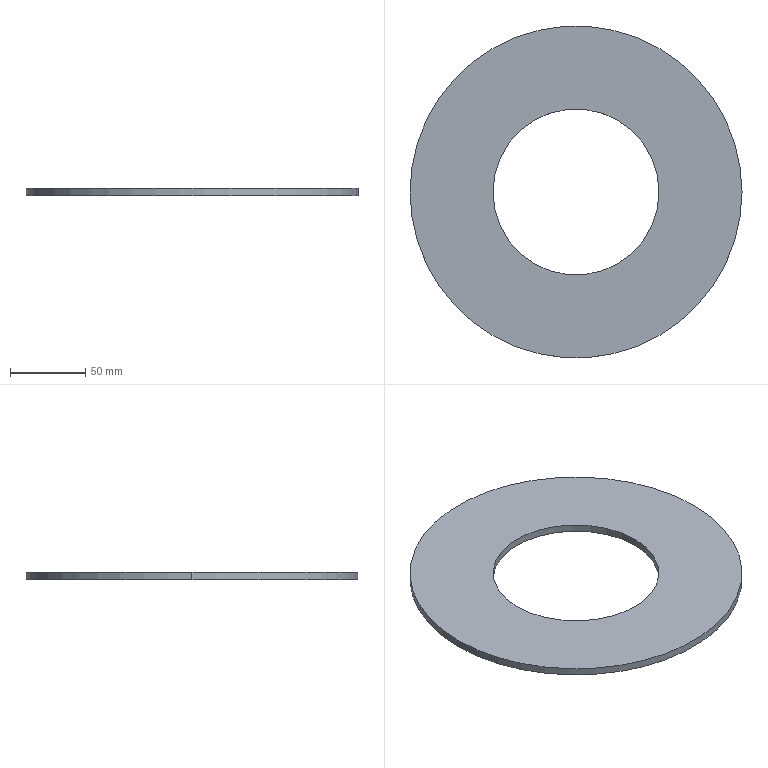Part | SolidWorks | features Extrusion 1 | 1 solid | 6 faces | box 220 x 220 x 5 mm | volume 142550 mm3 | cylinder 4 | plane 2 | commonest cylinder face diameters 110 x2 220 x2
STEP:
#1=CARTESIAN_POINT('',(-57.717,0.5838,5.));
#2=VERTEX_POINT('',#1);
#3=CARTESIAN_POINT('',(52.283,0.5838,5.));
#4=VERTEX_POINT('',#3);
#5=CARTESIAN_POINT('',(-2.717,0.5838,5.));
#6=DIRECTION('',(0.,0.,1.));
#7=DIRECTION('',(1.,0.,0.));
#8=AXIS2_PLACEMENT_3D('',#5,#6,#7);
#9=CIRCLE('',#8,55.);
#10=EDGE_CURVE('',#2,#4,#9,.T.);
#11=ORIENTED_EDGE('',*,*,#10,.T.);
#12=CARTESIAN_POINT('',(52.283,0.5838,0.));
#13=VERTEX_POINT('',#12);
#14=CARTESIAN_POINT('',(52.283,0.5838,5.));
#15=DIRECTION('',(0.,0.,-1.));
#16=VECTOR('',#15,1000.);
#17=LINE('',#14,#16);
#18=EDGE_CURVE('',#4,#13,#17,.T.);
#19=ORIENTED_EDGE('',*,*,#18,.T.);
#20=CARTESIAN_POINT('',(-57.717,0.5838,0.));
#21=VERTEX_POINT('',#20);
#22=CARTESIAN_POINT('',(-2.717,0.5838,0.));
#23=DIRECTION('',(0.,0.,1.));
#24=DIRECTION('',(1.,0.,0.));
#25=AXIS2_PLACEMENT_3D('',#22,#23,#24);
#26=CIRCLE('',#25,55.);
#27=EDGE_CURVE('',#21,#13,#26,.T.);
#28=ORIENTED_EDGE('',*,*,#27,.F.);
#29=CARTESIAN_POINT('',(-57.717,0.5838,5.));
#30=DIRECTION('',(0.,0.,-1.));
#31=VECTOR('',#30,1000.);
#32=LINE('',#29,#31);
#33=EDGE_CURVE('',#2,#21,#32,.T.);
#34=ORIENTED_EDGE('',*,*,#33,.F.);
#35=EDGE_LOOP('',(#11,#19,#28,#34));
#36=FACE_OUTER_BOUND('',#35,.T.);
#37=CARTESIAN_POINT('',(-2.717,0.5838,5.));
#38=DIRECTION('',(0.,0.,-1.));
#39=DIRECTION('',(-1.,0.,0.));
#40=AXIS2_PLACEMENT_3D('',#37,#38,#39);
#41=CYLINDRICAL_SURFACE('',#40,55.);
#42=ADVANCED_FACE('',(#36),#41,.F.);
#43=CARTESIAN_POINT('',(107.283,0.5838,5.));
#44=VERTEX_POINT('',#43);
#45=CARTESIAN_POINT('',(-112.717,0.5838,5.));
#46=VERTEX_POINT('',#45);
#47=CARTESIAN_POINT('',(-2.717,0.5838,5.));
#48=DIRECTION('',(0.,0.,1.));
#49=DIRECTION('',(1.,0.,0.));
#50=AXIS2_PLACEMENT_3D('',#47,#48,#49);
#51=CIRCLE('',#50,110.);
#52=EDGE_CURVE('',#44,#46,#51,.T.);
#53=ORIENTED_EDGE('',*,*,#52,.F.);
#54=CARTESIAN_POINT('',(107.283,0.5838,0.));
#55=VERTEX_POINT('',#54);
#56=CARTESIAN_POINT('',(107.283,0.5838,5.));
#57=DIRECTION('',(0.,0.,-1.));
#58=VECTOR('',#57,1000.);
#59=LINE('',#56,#58);
#60=EDGE_CURVE('',#44,#55,#59,.T.);
#61=ORIENTED_EDGE('',*,*,#60,.T.);
#62=CARTESIAN_POINT('',(-112.717,0.5838,0.));
#63=VERTEX_POINT('',#62);
#64=CARTESIAN_POINT('',(-2.717,0.5838,0.));
#65=DIRECTION('',(0.,0.,1.));
#66=DIRECTION('',(1.,0.,0.));
#67=AXIS2_PLACEMENT_3D('',#64,#65,#66);
#68=CIRCLE('',#67,110.);
#69=EDGE_CURVE('',#55,#63,#68,.T.);
#70=ORIENTED_EDGE('',*,*,#69,.T.);
#71=CARTESIAN_POINT('',(-112.717,0.5838,5.));
#72=DIRECTION('',(0.,0.,-1.));
#73=VECTOR('',#72,1000.);
#74=LINE('',#71,#73);
#75=EDGE_CURVE('',#46,#63,#74,.T.);
#76=ORIENTED_EDGE('',*,*,#75,.F.);
#77=EDGE_LOOP('',(#53,#61,#70,#76));
#78=FACE_OUTER_BOUND('',#77,.T.);
#79=CARTESIAN_POINT('',(-2.717,0.5838,5.));
#80=DIRECTION('',(0.,0.,-1.));
#81=DIRECTION('',(-1.,0.,0.));
#82=AXIS2_PLACEMENT_3D('',#79,#80,#81);
#83=CYLINDRICAL_SURFACE('',#82,110.);
#84=ADVANCED_FACE('',(#78),#83,.T.);
#85=CARTESIAN_POINT('',(-2.717,0.5838,5.));
#86=DIRECTION('',(0.,0.,1.));
#87=DIRECTION('',(1.,0.,0.));
#88=AXIS2_PLACEMENT_3D('',#85,#86,#87);
#89=CIRCLE('',#88,110.);
#90=EDGE_CURVE('',#46,#44,#89,.T.);
#91=ORIENTED_EDGE('',*,*,#90,.T.);
#92=ORIENTED_EDGE('',*,*,#52,.T.);
#93=EDGE_LOOP('',(#91,#92));
#94=FACE_OUTER_BOUND('',#93,.T.);
#95=ORIENTED_EDGE('',*,*,#10,.F.);
#96=CARTESIAN_POINT('',(-2.717,0.5838,5.));
#97=DIRECTION('',(0.,0.,1.));
#98=DIRECTION('',(1.,0.,0.));
#99=AXIS2_PLACEMENT_3D('',#96,#97,#98);
#100=CIRCLE('',#99,55.);
#101=EDGE_CURVE('',#4,#2,#100,.T.);
#102=ORIENTED_EDGE('',*,*,#101,.F.);
#103=EDGE_LOOP('',(#95,#102));
#104=FACE_BOUND('',#103,.T.);
#105=CARTESIAN_POINT('',(-2.717,0.5838,5.));
#106=DIRECTION('',(0.,0.,1.));
#107=DIRECTION('',(1.,0.,0.));
#108=AXIS2_PLACEMENT_3D('',#105,#106,#107);
#109=PLANE('',#108);
#110=ADVANCED_FACE('',(#94,#104),#109,.T.);
#111=CARTESIAN_POINT('',(-2.717,0.5838,0.));
#112=DIRECTION('',(0.,0.,1.));
#113=DIRECTION('',(1.,0.,0.));
#114=AXIS2_PLACEMENT_3D('',#111,#112,#113);
#115=CIRCLE('',#114,110.);
#116=EDGE_CURVE('',#63,#55,#115,.T.);
#117=ORIENTED_EDGE('',*,*,#116,.F.);
#118=ORIENTED_EDGE('',*,*,#69,.F.);
#119=EDGE_LOOP('',(#117,#118));
#120=FACE_OUTER_BOUND('',#119,.T.);
#121=ORIENTED_EDGE('',*,*,#27,.T.);
#122=CARTESIAN_POINT('',(-2.717,0.5838,0.));
#123=DIRECTION('',(0.,0.,1.));
#124=DIRECTION('',(1.,0.,0.));
#125=AXIS2_PLACEMENT_3D('',#122,#123,#124);
#126=CIRCLE('',#125,55.);
#127=EDGE_CURVE('',#13,#21,#126,.T.);
#128=ORIENTED_EDGE('',*,*,#127,.T.);
#129=EDGE_LOOP('',(#121,#128));
#130=FACE_BOUND('',#129,.T.);
#131=CARTESIAN_POINT('',(-2.717,0.5838,0.));
#132=DIRECTION('',(0.,0.,1.));
#133=DIRECTION('',(1.,0.,0.));
#134=AXIS2_PLACEMENT_3D('',#131,#132,#133);
#135=PLANE('',#134);
#136=ADVANCED_FACE('',(#120,#130),#135,.F.);
#137=ORIENTED_EDGE('',*,*,#60,.F.);
#138=ORIENTED_EDGE('',*,*,#90,.F.);
#139=ORIENTED_EDGE('',*,*,#75,.T.);
#140=ORIENTED_EDGE('',*,*,#116,.T.);
#141=EDGE_LOOP('',(#137,#138,#139,#140));
#142=FACE_OUTER_BOUND('',#141,.T.);
#143=CARTESIAN_POINT('',(-2.717,0.5838,5.));
#144=DIRECTION('',(0.,0.,-1.));
#145=DIRECTION('',(-1.,0.,0.));
#146=AXIS2_PLACEMENT_3D('',#143,#144,#145);
#147=CYLINDRICAL_SURFACE('',#146,110.);
#148=ADVANCED_FACE('',(#142),#147,.T.);
#149=ORIENTED_EDGE('',*,*,#18,.F.);
#150=ORIENTED_EDGE('',*,*,#101,.T.);
#151=ORIENTED_EDGE('',*,*,#33,.T.);
#152=ORIENTED_EDGE('',*,*,#127,.F.);
#153=EDGE_LOOP('',(#149,#150,#151,#152));
#154=FACE_OUTER_BOUND('',#153,.T.);
#155=CARTESIAN_POINT('',(-2.717,0.5838,5.));
#156=DIRECTION('',(0.,0.,-1.));
#157=DIRECTION('',(-1.,0.,0.));
#158=AXIS2_PLACEMENT_3D('',#155,#156,#157);
#159=CYLINDRICAL_SURFACE('',#158,55.);
#160=ADVANCED_FACE('',(#154),#159,.F.);
#161=CLOSED_SHELL('',(#42,#84,#110,#136,#148,#160));
#162=MANIFOLD_SOLID_BREP('',#161);
#163=CARTESIAN_POINT('',(0.,0.,0.));
#164=DIRECTION('',(0.,0.,1.));
#165=DIRECTION('',(1.,0.,0.));
#166=AXIS2_PLACEMENT_3D('',#163,#164,#165);
#167=(LENGTH_UNIT()NAMED_UNIT(*)SI_UNIT(.MILLI.,.METRE.));
#168=UNCERTAINTY_MEASURE_WITH_UNIT(LENGTH_MEASURE(0.00001),#167,'','');
#169=(NAMED_UNIT(*)PLANE_ANGLE_UNIT()SI_UNIT($,.RADIAN.));
#170=(NAMED_UNIT(*)SI_UNIT($,.STERADIAN.)SOLID_ANGLE_UNIT());
#171=(GEOMETRIC_REPRESENTATION_CONTEXT(3)GLOBAL_UNCERTAINTY_ASSIGNED_CONTEXT((#168))GLOBAL_UNIT_ASSIGNED_CONTEXT((#167,#169,#170))REPRESENTATION_CONTEXT('',''));
#172=ADVANCED_BREP_SHAPE_REPRESENTATION('',(#162,#166),#171);